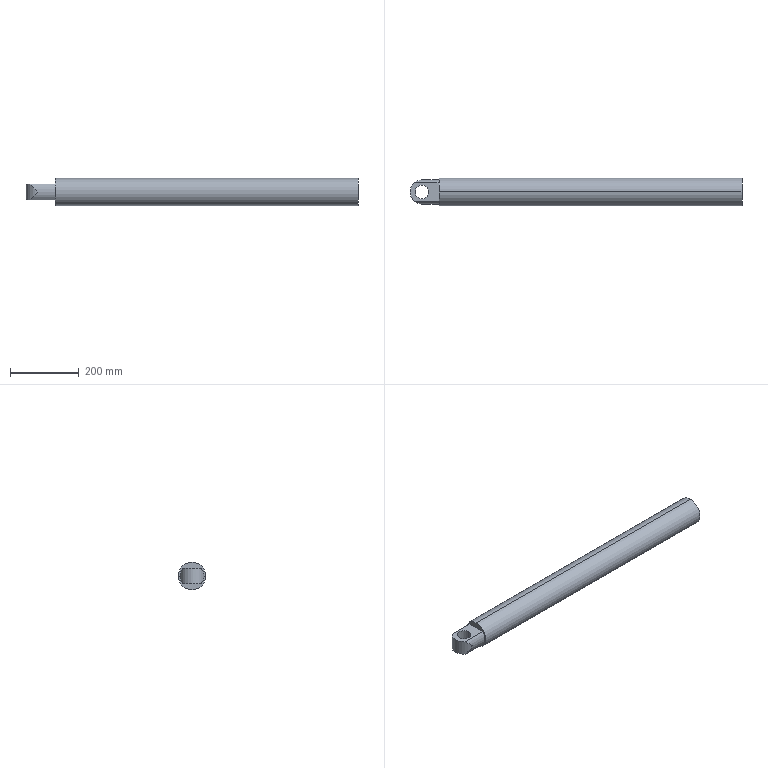Part | SolidWorks | features ICE 2, Revolution 1 | 1 solid | 14 faces | box 968 x 80 x 80 mm | volume 3418828 mm3 | cylinder 9 | plane 5 | commonest cylinder face diameters 70 x3 40 x2 45 x2 80 x2
STEP:
#1=CARTESIAN_POINT('',(-953.,0.,-22.5));
#2=VERTEX_POINT('',#1);
#3=CARTESIAN_POINT('',(-913.,0.,-22.5));
#4=VERTEX_POINT('',#3);
#5=CARTESIAN_POINT('',(-933.,0.,-22.5));
#6=DIRECTION('',(0.,0.,1.));
#7=DIRECTION('',(-1.,0.,0.));
#8=AXIS2_PLACEMENT_3D('',#5,#6,#7);
#9=CIRCLE('',#8,20.);
#10=EDGE_CURVE('',#2,#4,#9,.T.);
#11=ORIENTED_EDGE('',*,*,#10,.F.);
#12=CARTESIAN_POINT('',(-953.,0.,22.5));
#13=VERTEX_POINT('',#12);
#14=CARTESIAN_POINT('',(-953.,0.,-40.));
#15=DIRECTION('',(0.,0.,1.));
#16=VECTOR('',#15,1000.);
#17=LINE('',#14,#16);
#18=EDGE_CURVE('',#2,#13,#17,.T.);
#19=ORIENTED_EDGE('',*,*,#18,.T.);
#20=CARTESIAN_POINT('',(-913.,0.,22.5));
#21=VERTEX_POINT('',#20);
#22=CARTESIAN_POINT('',(-933.,0.,22.5));
#23=DIRECTION('',(0.,0.,-1.));
#24=DIRECTION('',(1.,0.,0.));
#25=AXIS2_PLACEMENT_3D('',#22,#23,#24);
#26=CIRCLE('',#25,20.);
#27=EDGE_CURVE('',#21,#13,#26,.T.);
#28=ORIENTED_EDGE('',*,*,#27,.F.);
#29=CARTESIAN_POINT('',(-913.,0.,-40.));
#30=DIRECTION('',(0.,0.,1.));
#31=VECTOR('',#30,1000.);
#32=LINE('',#29,#31);
#33=EDGE_CURVE('',#4,#21,#32,.T.);
#34=ORIENTED_EDGE('',*,*,#33,.F.);
#35=EDGE_LOOP('',(#11,#19,#28,#34));
#36=FACE_OUTER_BOUND('',#35,.T.);
#37=CARTESIAN_POINT('',(-933.,0.,-40.));
#38=DIRECTION('',(0.,0.,1.));
#39=DIRECTION('',(1.,0.,0.));
#40=AXIS2_PLACEMENT_3D('',#37,#38,#39);
#41=CYLINDRICAL_SURFACE('',#40,20.);
#42=ADVANCED_FACE('',(#36),#41,.F.);
#43=CARTESIAN_POINT('',(0.,0.,40.));
#44=VERTEX_POINT('',#43);
#45=CARTESIAN_POINT('',(0.,0.,-40.));
#46=VERTEX_POINT('',#45);
#47=CARTESIAN_POINT('',(0.,0.,0.));
#48=DIRECTION('',(-1.,0.,0.));
#49=DIRECTION('',(0.,0.,1.));
#50=AXIS2_PLACEMENT_3D('',#47,#48,#49);
#51=CIRCLE('',#50,40.);
#52=EDGE_CURVE('',#44,#46,#51,.T.);
#53=ORIENTED_EDGE('',*,*,#52,.T.);
#54=CARTESIAN_POINT('',(-883.,0.,-40.));
#55=VERTEX_POINT('',#54);
#56=CARTESIAN_POINT('',(-802.168,0.,-40.));
#57=DIRECTION('',(-1.,0.,0.));
#58=VECTOR('',#57,1000.);
#59=LINE('',#56,#58);
#60=EDGE_CURVE('',#46,#55,#59,.T.);
#61=ORIENTED_EDGE('',*,*,#60,.T.);
#62=CARTESIAN_POINT('',(-883.,0.,40.));
#63=VERTEX_POINT('',#62);
#64=CARTESIAN_POINT('',(-883.,0.,0.));
#65=DIRECTION('',(-1.,0.,0.));
#66=DIRECTION('',(0.,0.,1.));
#67=AXIS2_PLACEMENT_3D('',#64,#65,#66);
#68=CIRCLE('',#67,40.);
#69=EDGE_CURVE('',#63,#55,#68,.T.);
#70=ORIENTED_EDGE('',*,*,#69,.F.);
#71=CARTESIAN_POINT('',(-802.168,0.,40.));
#72=DIRECTION('',(-1.,0.,0.));
#73=VECTOR('',#72,1000.);
#74=LINE('',#71,#73);
#75=EDGE_CURVE('',#44,#63,#74,.T.);
#76=ORIENTED_EDGE('',*,*,#75,.F.);
#77=EDGE_LOOP('',(#53,#61,#70,#76));
#78=FACE_OUTER_BOUND('',#77,.T.);
#79=CARTESIAN_POINT('',(-802.168,0.,0.));
#80=DIRECTION('',(-1.,0.,0.));
#81=DIRECTION('',(0.,0.,1.));
#82=AXIS2_PLACEMENT_3D('',#79,#80,#81);
#83=CYLINDRICAL_SURFACE('',#82,40.);
#84=ADVANCED_FACE('',(#78),#83,.T.);
#85=CARTESIAN_POINT('',(0.,0.,-22.5));
#86=VERTEX_POINT('',#85);
#87=CARTESIAN_POINT('',(0.,0.,22.5));
#88=VERTEX_POINT('',#87);
#89=CARTESIAN_POINT('',(0.,0.,0.));
#90=DIRECTION('',(-1.,0.,0.));
#91=DIRECTION('',(0.,0.,1.));
#92=AXIS2_PLACEMENT_3D('',#89,#90,#91);
#93=CIRCLE('',#92,22.5);
#94=EDGE_CURVE('',#86,#88,#93,.T.);
#95=ORIENTED_EDGE('',*,*,#94,.F.);
#96=CARTESIAN_POINT('',(-750.,0.,-22.5));
#97=VERTEX_POINT('',#96);
#98=CARTESIAN_POINT('',(-802.168,0.,-22.5));
#99=DIRECTION('',(-1.,0.,0.));
#100=VECTOR('',#99,1000.);
#101=LINE('',#98,#100);
#102=EDGE_CURVE('',#86,#97,#101,.T.);
#103=ORIENTED_EDGE('',*,*,#102,.T.);
#104=CARTESIAN_POINT('',(-750.,0.,22.5));
#105=VERTEX_POINT('',#104);
#106=CARTESIAN_POINT('',(-750.,0.,0.));
#107=DIRECTION('',(-1.,0.,0.));
#108=DIRECTION('',(0.,0.,1.));
#109=AXIS2_PLACEMENT_3D('',#106,#107,#108);
#110=CIRCLE('',#109,22.5);
#111=EDGE_CURVE('',#97,#105,#110,.T.);
#112=ORIENTED_EDGE('',*,*,#111,.T.);
#113=CARTESIAN_POINT('',(-802.168,0.,22.5));
#114=DIRECTION('',(-1.,0.,0.));
#115=VECTOR('',#114,1000.);
#116=LINE('',#113,#115);
#117=EDGE_CURVE('',#88,#105,#116,.T.);
#118=ORIENTED_EDGE('',*,*,#117,.F.);
#119=EDGE_LOOP('',(#95,#103,#112,#118));
#120=FACE_OUTER_BOUND('',#119,.T.);
#121=CARTESIAN_POINT('',(-802.168,0.,0.));
#122=DIRECTION('',(-1.,0.,0.));
#123=DIRECTION('',(0.,0.,1.));
#124=AXIS2_PLACEMENT_3D('',#121,#122,#123);
#125=CYLINDRICAL_SURFACE('',#124,22.5);
#126=ADVANCED_FACE('',(#120),#125,.F.);
#127=CARTESIAN_POINT('',(-883.,-26.81,-22.5));
#128=VERTEX_POINT('',#127);
#129=CARTESIAN_POINT('',(-955.5,-26.81,-22.5));
#130=VERTEX_POINT('',#129);
#131=CARTESIAN_POINT('',(-802.168,-26.81,-22.5));
#132=DIRECTION('',(-1.,0.,0.));
#133=VECTOR('',#132,1000.);
#134=LINE('',#131,#133);
#135=EDGE_CURVE('',#128,#130,#134,.T.);
#136=ORIENTED_EDGE('',*,*,#135,.F.);
#137=CARTESIAN_POINT('',(-883.,-26.81,22.5));
#138=VERTEX_POINT('',#137);
#139=CARTESIAN_POINT('',(-883.,0.,0.));
#140=DIRECTION('',(-1.,0.,0.));
#141=DIRECTION('',(0.,0.,1.));
#142=AXIS2_PLACEMENT_3D('',#139,#140,#141);
#143=CIRCLE('',#142,35.);
#144=EDGE_CURVE('',#128,#138,#143,.T.);
#145=ORIENTED_EDGE('',*,*,#144,.T.);
#146=CARTESIAN_POINT('',(-955.5,-26.81,22.5));
#147=VERTEX_POINT('',#146);
#148=CARTESIAN_POINT('',(-802.168,-26.81,22.5));
#149=DIRECTION('',(1.,0.,0.));
#150=VECTOR('',#149,1000.);
#151=LINE('',#148,#150);
#152=EDGE_CURVE('',#147,#138,#151,.T.);
#153=ORIENTED_EDGE('',*,*,#152,.F.);
#154=CARTESIAN_POINT('',(-933.,-35.,0.));
#155=VERTEX_POINT('',#154);
#156=CARTESIAN_POINT('',(-933.,-35.,0.));
#157=CARTESIAN_POINT('',(-941.316,-35.,8.316));
#158=CARTESIAN_POINT('',(-949.13,-32.155,16.13));
#159=CARTESIAN_POINT('',(-955.5,-26.81,22.5));
#160=(BOUNDED_CURVE()B_SPLINE_CURVE(3,(#156,#157,#158,#159),.UNSPECIFIED.,.F.,.F.)B_SPLINE_CURVE_WITH_KNOTS((4,4),(4.712,5.411),.UNSPECIFIED.)CURVE()GEOMETRIC_REPRESENTATION_ITEM()RATIONAL_B_SPLINE_CURVE((1.,0.9598,0.9598,1.))REPRESENTATION_ITEM(''));
#161=EDGE_CURVE('',#155,#147,#160,.T.);
#162=ORIENTED_EDGE('',*,*,#161,.F.);
#163=CARTESIAN_POINT('',(-955.5,-26.81,-22.5));
#164=CARTESIAN_POINT('',(-949.13,-32.155,-16.13));
#165=CARTESIAN_POINT('',(-941.316,-35.,-8.316));
#166=CARTESIAN_POINT('',(-933.,-35.,0.));
#167=(BOUNDED_CURVE()B_SPLINE_CURVE(3,(#163,#164,#165,#166),.UNSPECIFIED.,.F.,.T.)B_SPLINE_CURVE_WITH_KNOTS((4,4),(0.8726,1.571),.UNSPECIFIED.)CURVE()GEOMETRIC_REPRESENTATION_ITEM()RATIONAL_B_SPLINE_CURVE((1.,0.9598,0.9598,1.))REPRESENTATION_ITEM(''));
#168=EDGE_CURVE('',#130,#155,#167,.T.);
#169=ORIENTED_EDGE('',*,*,#168,.F.);
#170=EDGE_LOOP('',(#136,#145,#153,#162,#169));
#171=FACE_OUTER_BOUND('',#170,.T.);
#172=CARTESIAN_POINT('',(-802.168,0.,0.));
#173=DIRECTION('',(-1.,0.,0.));
#174=DIRECTION('',(0.,0.,1.));
#175=AXIS2_PLACEMENT_3D('',#172,#173,#174);
#176=CYLINDRICAL_SURFACE('',#175,35.);
#177=ADVANCED_FACE('',(#171),#176,.T.);
#178=CARTESIAN_POINT('',(-955.5,26.81,-22.5));
#179=VERTEX_POINT('',#178);
#180=CARTESIAN_POINT('',(-883.,26.81,-22.5));
#181=VERTEX_POINT('',#180);
#182=CARTESIAN_POINT('',(-802.168,26.81,-22.5));
#183=DIRECTION('',(1.,0.,0.));
#184=VECTOR('',#183,1000.);
#185=LINE('',#182,#184);
#186=EDGE_CURVE('',#179,#181,#185,.T.);
#187=ORIENTED_EDGE('',*,*,#186,.F.);
#188=CARTESIAN_POINT('',(-933.,35.,0.));
#189=VERTEX_POINT('',#188);
#190=CARTESIAN_POINT('',(-933.,35.,0.));
#191=CARTESIAN_POINT('',(-941.316,35.,-8.316));
#192=CARTESIAN_POINT('',(-949.13,32.155,-16.13));
#193=CARTESIAN_POINT('',(-955.5,26.81,-22.5));
#194=(BOUNDED_CURVE()B_SPLINE_CURVE(3,(#190,#191,#192,#193),.UNSPECIFIED.,.F.,.F.)B_SPLINE_CURVE_WITH_KNOTS((4,4),(4.712,5.411),.UNSPECIFIED.)CURVE()GEOMETRIC_REPRESENTATION_ITEM()RATIONAL_B_SPLINE_CURVE((1.,0.9598,0.9598,1.))REPRESENTATION_ITEM(''));
#195=EDGE_CURVE('',#189,#179,#194,.T.);
#196=ORIENTED_EDGE('',*,*,#195,.F.);
#197=CARTESIAN_POINT('',(-955.5,26.81,22.5));
#198=VERTEX_POINT('',#197);
#199=CARTESIAN_POINT('',(-955.5,26.81,22.5));
#200=CARTESIAN_POINT('',(-949.13,32.155,16.13));
#201=CARTESIAN_POINT('',(-941.316,35.,8.316));
#202=CARTESIAN_POINT('',(-933.,35.,0.));
#203=(BOUNDED_CURVE()B_SPLINE_CURVE(3,(#199,#200,#201,#202),.UNSPECIFIED.,.F.,.F.)B_SPLINE_CURVE_WITH_KNOTS((4,4),(0.8726,1.571),.UNSPECIFIED.)CURVE()GEOMETRIC_REPRESENTATION_ITEM()RATIONAL_B_SPLINE_CURVE((1.,0.9598,0.9598,1.))REPRESENTATION_ITEM(''));
#204=EDGE_CURVE('',#198,#189,#203,.T.);
#205=ORIENTED_EDGE('',*,*,#204,.F.);
#206=CARTESIAN_POINT('',(-883.,26.81,22.5));
#207=VERTEX_POINT('',#206);
#208=CARTESIAN_POINT('',(-802.168,26.81,22.5));
#209=DIRECTION('',(-1.,0.,0.));
#210=VECTOR('',#209,1000.);
#211=LINE('',#208,#210);
#212=EDGE_CURVE('',#207,#198,#211,.T.);
#213=ORIENTED_EDGE('',*,*,#212,.F.);
#214=CARTESIAN_POINT('',(-883.,0.,0.));
#215=DIRECTION('',(-1.,0.,0.));
#216=DIRECTION('',(0.,0.,1.));
#217=AXIS2_PLACEMENT_3D('',#214,#215,#216);
#218=CIRCLE('',#217,35.);
#219=EDGE_CURVE('',#207,#181,#218,.T.);
#220=ORIENTED_EDGE('',*,*,#219,.T.);
#221=EDGE_LOOP('',(#187,#196,#205,#213,#220));
#222=FACE_OUTER_BOUND('',#221,.T.);
#223=CARTESIAN_POINT('',(-802.168,0.,0.));
#224=DIRECTION('',(-1.,0.,0.));
#225=DIRECTION('',(0.,0.,1.));
#226=AXIS2_PLACEMENT_3D('',#223,#224,#225);
#227=CYLINDRICAL_SURFACE('',#226,35.);
#228=ADVANCED_FACE('',(#222),#227,.T.);
#229=CARTESIAN_POINT('',(-933.,0.,-22.5));
#230=DIRECTION('',(0.,0.,1.));
#231=DIRECTION('',(-1.,0.,0.));
#232=AXIS2_PLACEMENT_3D('',#229,#230,#231);
#233=CIRCLE('',#232,35.);
#234=EDGE_CURVE('',#179,#130,#233,.T.);
#235=ORIENTED_EDGE('',*,*,#234,.T.);
#236=ORIENTED_EDGE('',*,*,#168,.T.);
#237=ORIENTED_EDGE('',*,*,#161,.T.);
#238=CARTESIAN_POINT('',(-933.,0.,22.5));
#239=DIRECTION('',(0.,0.,-1.));
#240=DIRECTION('',(1.,0.,0.));
#241=AXIS2_PLACEMENT_3D('',#238,#239,#240);
#242=CIRCLE('',#241,35.);
#243=EDGE_CURVE('',#147,#198,#242,.T.);
#244=ORIENTED_EDGE('',*,*,#243,.T.);
#245=ORIENTED_EDGE('',*,*,#204,.T.);
#246=ORIENTED_EDGE('',*,*,#195,.T.);
#247=EDGE_LOOP('',(#235,#236,#237,#244,#245,#246));
#248=FACE_OUTER_BOUND('',#247,.T.);
#249=CARTESIAN_POINT('',(-933.,0.,-40.));
#250=DIRECTION('',(0.,0.,1.));
#251=DIRECTION('',(1.,0.,0.));
#252=AXIS2_PLACEMENT_3D('',#249,#250,#251);
#253=CYLINDRICAL_SURFACE('',#252,35.);
#254=ADVANCED_FACE('',(#248),#253,.T.);
#255=ORIENTED_EDGE('',*,*,#52,.F.);
#256=CARTESIAN_POINT('',(0.,0.,0.));
#257=DIRECTION('',(-1.,0.,0.));
#258=DIRECTION('',(0.,0.,1.));
#259=AXIS2_PLACEMENT_3D('',#256,#257,#258);
#260=CIRCLE('',#259,40.);
#261=EDGE_CURVE('',#46,#44,#260,.T.);
#262=ORIENTED_EDGE('',*,*,#261,.F.);
#263=EDGE_LOOP('',(#255,#262));
#264=FACE_OUTER_BOUND('',#263,.T.);
#265=CARTESIAN_POINT('',(0.,0.,0.));
#266=DIRECTION('',(-1.,0.,0.));
#267=DIRECTION('',(0.,0.,1.));
#268=AXIS2_PLACEMENT_3D('',#265,#266,#267);
#269=CIRCLE('',#268,22.5);
#270=EDGE_CURVE('',#88,#86,#269,.T.);
#271=ORIENTED_EDGE('',*,*,#270,.T.);
#272=ORIENTED_EDGE('',*,*,#94,.T.);
#273=EDGE_LOOP('',(#271,#272));
#274=FACE_BOUND('',#273,.T.);
#275=CARTESIAN_POINT('',(0.,40.,0.));
#276=DIRECTION('',(-1.,0.,0.));
#277=DIRECTION('',(0.,0.,1.));
#278=AXIS2_PLACEMENT_3D('',#275,#276,#277);
#279=PLANE('',#278);
#280=ADVANCED_FACE('',(#264,#274),#279,.F.);
#281=ORIENTED_EDGE('',*,*,#102,.F.);
#282=ORIENTED_EDGE('',*,*,#270,.F.);
#283=ORIENTED_EDGE('',*,*,#117,.T.);
#284=CARTESIAN_POINT('',(-750.,0.,0.));
#285=DIRECTION('',(-1.,0.,0.));
#286=DIRECTION('',(0.,0.,1.));
#287=AXIS2_PLACEMENT_3D('',#284,#285,#286);
#288=CIRCLE('',#287,22.5);
#289=EDGE_CURVE('',#105,#97,#288,.T.);
#290=ORIENTED_EDGE('',*,*,#289,.T.);
#291=EDGE_LOOP('',(#281,#282,#283,#290));
#292=FACE_OUTER_BOUND('',#291,.T.);
#293=CARTESIAN_POINT('',(-802.168,0.,0.));
#294=DIRECTION('',(-1.,0.,0.));
#295=DIRECTION('',(0.,0.,1.));
#296=AXIS2_PLACEMENT_3D('',#293,#294,#295);
#297=CYLINDRICAL_SURFACE('',#296,22.5);
#298=ADVANCED_FACE('',(#292),#297,.F.);
#299=ORIENTED_EDGE('',*,*,#289,.F.);
#300=ORIENTED_EDGE('',*,*,#111,.F.);
#301=EDGE_LOOP('',(#299,#300));
#302=FACE_OUTER_BOUND('',#301,.T.);
#303=CARTESIAN_POINT('',(-750.,22.5,0.));
#304=DIRECTION('',(-1.,0.,0.));
#305=DIRECTION('',(0.,0.,1.));
#306=AXIS2_PLACEMENT_3D('',#303,#304,#305);
#307=PLANE('',#306);
#308=ADVANCED_FACE('',(#302),#307,.F.);
#309=ORIENTED_EDGE('',*,*,#144,.F.);
#310=CARTESIAN_POINT('',(-883.,50.,-22.5));
#311=DIRECTION('',(0.,1.,0.));
#312=VECTOR('',#311,1000.);
#313=LINE('',#310,#312);
#314=EDGE_CURVE('',#128,#181,#313,.T.);
#315=ORIENTED_EDGE('',*,*,#314,.T.);
#316=ORIENTED_EDGE('',*,*,#219,.F.);
#317=CARTESIAN_POINT('',(-883.,50.,22.5));
#318=DIRECTION('',(0.,-1.,0.));
#319=VECTOR('',#318,1000.);
#320=LINE('',#317,#319);
#321=EDGE_CURVE('',#207,#138,#320,.T.);
#322=ORIENTED_EDGE('',*,*,#321,.T.);
#323=EDGE_LOOP('',(#309,#315,#316,#322));
#324=FACE_BOUND('',#323,.T.);
#325=ORIENTED_EDGE('',*,*,#69,.T.);
#326=CARTESIAN_POINT('',(-883.,0.,0.));
#327=DIRECTION('',(-1.,0.,0.));
#328=DIRECTION('',(0.,0.,1.));
#329=AXIS2_PLACEMENT_3D('',#326,#327,#328);
#330=CIRCLE('',#329,40.);
#331=EDGE_CURVE('',#55,#63,#330,.T.);
#332=ORIENTED_EDGE('',*,*,#331,.T.);
#333=EDGE_LOOP('',(#325,#332));
#334=FACE_OUTER_BOUND('',#333,.T.);
#335=CARTESIAN_POINT('',(-883.,40.,0.));
#336=DIRECTION('',(1.,0.,0.));
#337=DIRECTION('',(0.,0.,-1.));
#338=AXIS2_PLACEMENT_3D('',#335,#336,#337);
#339=PLANE('',#338);
#340=ADVANCED_FACE('',(#324,#334),#339,.F.);
#341=ORIENTED_EDGE('',*,*,#60,.F.);
#342=ORIENTED_EDGE('',*,*,#261,.T.);
#343=ORIENTED_EDGE('',*,*,#75,.T.);
#344=ORIENTED_EDGE('',*,*,#331,.F.);
#345=EDGE_LOOP('',(#341,#342,#343,#344));
#346=FACE_OUTER_BOUND('',#345,.T.);
#347=CARTESIAN_POINT('',(-802.168,0.,0.));
#348=DIRECTION('',(-1.,0.,0.));
#349=DIRECTION('',(0.,0.,1.));
#350=AXIS2_PLACEMENT_3D('',#347,#348,#349);
#351=CYLINDRICAL_SURFACE('',#350,40.);
#352=ADVANCED_FACE('',(#346),#351,.T.);
#353=ORIENTED_EDGE('',*,*,#212,.T.);
#354=ORIENTED_EDGE('',*,*,#243,.F.);
#355=ORIENTED_EDGE('',*,*,#152,.T.);
#356=ORIENTED_EDGE('',*,*,#321,.F.);
#357=EDGE_LOOP('',(#353,#354,#355,#356));
#358=FACE_OUTER_BOUND('',#357,.T.);
#359=ORIENTED_EDGE('',*,*,#27,.T.);
#360=CARTESIAN_POINT('',(-933.,0.,22.5));
#361=DIRECTION('',(0.,0.,-1.));
#362=DIRECTION('',(1.,0.,0.));
#363=AXIS2_PLACEMENT_3D('',#360,#361,#362);
#364=CIRCLE('',#363,20.);
#365=EDGE_CURVE('',#13,#21,#364,.T.);
#366=ORIENTED_EDGE('',*,*,#365,.T.);
#367=EDGE_LOOP('',(#359,#366));
#368=FACE_BOUND('',#367,.T.);
#369=CARTESIAN_POINT('',(-968.,50.,22.5));
#370=DIRECTION('',(0.,0.,1.));
#371=DIRECTION('',(1.,0.,0.));
#372=AXIS2_PLACEMENT_3D('',#369,#370,#371);
#373=PLANE('',#372);
#374=ADVANCED_FACE('',(#358,#368),#373,.T.);
#375=ORIENTED_EDGE('',*,*,#135,.T.);
#376=ORIENTED_EDGE('',*,*,#234,.F.);
#377=ORIENTED_EDGE('',*,*,#186,.T.);
#378=ORIENTED_EDGE('',*,*,#314,.F.);
#379=EDGE_LOOP('',(#375,#376,#377,#378));
#380=FACE_OUTER_BOUND('',#379,.T.);
#381=CARTESIAN_POINT('',(-933.,0.,-22.5));
#382=DIRECTION('',(0.,0.,1.));
#383=DIRECTION('',(-1.,0.,0.));
#384=AXIS2_PLACEMENT_3D('',#381,#382,#383);
#385=CIRCLE('',#384,20.);
#386=EDGE_CURVE('',#4,#2,#385,.T.);
#387=ORIENTED_EDGE('',*,*,#386,.T.);
#388=ORIENTED_EDGE('',*,*,#10,.T.);
#389=EDGE_LOOP('',(#387,#388));
#390=FACE_BOUND('',#389,.T.);
#391=CARTESIAN_POINT('',(-968.,50.,-22.5));
#392=DIRECTION('',(0.,0.,-1.));
#393=DIRECTION('',(-1.,0.,0.));
#394=AXIS2_PLACEMENT_3D('',#391,#392,#393);
#395=PLANE('',#394);
#396=ADVANCED_FACE('',(#380,#390),#395,.T.);
#397=ORIENTED_EDGE('',*,*,#18,.F.);
#398=ORIENTED_EDGE('',*,*,#386,.F.);
#399=ORIENTED_EDGE('',*,*,#33,.T.);
#400=ORIENTED_EDGE('',*,*,#365,.F.);
#401=EDGE_LOOP('',(#397,#398,#399,#400));
#402=FACE_OUTER_BOUND('',#401,.T.);
#403=CARTESIAN_POINT('',(-933.,0.,-40.));
#404=DIRECTION('',(0.,0.,1.));
#405=DIRECTION('',(1.,0.,0.));
#406=AXIS2_PLACEMENT_3D('',#403,#404,#405);
#407=CYLINDRICAL_SURFACE('',#406,20.);
#408=ADVANCED_FACE('',(#402),#407,.F.);
#409=CLOSED_SHELL('',(#42,#84,#126,#177,#228,#254,#280,#298,#308,#340,#352,#374,#396,#408));
#410=MANIFOLD_SOLID_BREP('',#409);
#411=CARTESIAN_POINT('',(0.,0.,0.));
#412=DIRECTION('',(0.,0.,1.));
#413=DIRECTION('',(1.,0.,0.));
#414=AXIS2_PLACEMENT_3D('',#411,#412,#413);
#415=(LENGTH_UNIT()NAMED_UNIT(*)SI_UNIT(.MILLI.,.METRE.));
#416=UNCERTAINTY_MEASURE_WITH_UNIT(LENGTH_MEASURE(0.00001),#415,'','');
#417=(NAMED_UNIT(*)PLANE_ANGLE_UNIT()SI_UNIT($,.RADIAN.));
#418=(NAMED_UNIT(*)SI_UNIT($,.STERADIAN.)SOLID_ANGLE_UNIT());
#419=(GEOMETRIC_REPRESENTATION_CONTEXT(3)GLOBAL_UNCERTAINTY_ASSIGNED_CONTEXT((#416))GLOBAL_UNIT_ASSIGNED_CONTEXT((#415,#417,#418))REPRESENTATION_CONTEXT('',''));
#420=ADVANCED_BREP_SHAPE_REPRESENTATION('',(#410,#414),#419);